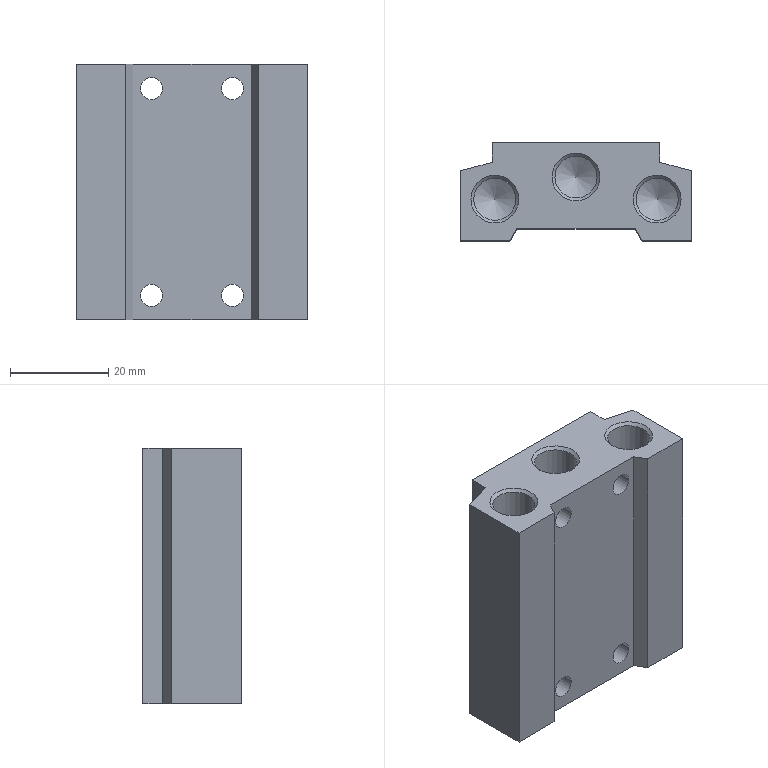Part | NX | 1 solid | 36 faces | box 47 x 20 x 52 mm | volume 37879 mm3 | plane 14 | cone 12 | cylinder 10 | commonest cylinder face diameters 8.566 x6 4.5 x4
STEP:
#1=CARTESIAN_POINT('',(-40.5,20.,0.));
#2=VERTEX_POINT('',#1);
#3=CARTESIAN_POINT('',(-6.5,20.,0.));
#4=VERTEX_POINT('',#3);
#5=CARTESIAN_POINT('',(-6.5,20.,0.));
#6=DIRECTION('',(1.,0.,0.));
#7=VECTOR('',#6,1000.);
#8=LINE('',#5,#7);
#9=EDGE_CURVE('',#2,#4,#8,.T.);
#10=ORIENTED_EDGE('',*,*,#9,.T.);
#11=CARTESIAN_POINT('',(-6.5,20.,-52.));
#12=VERTEX_POINT('',#11);
#13=CARTESIAN_POINT('',(-6.5,20.,0.));
#14=DIRECTION('',(0.,0.,1.));
#15=VECTOR('',#14,1000.);
#16=LINE('',#13,#15);
#17=EDGE_CURVE('',#4,#12,#16,.F.);
#18=ORIENTED_EDGE('',*,*,#17,.T.);
#19=CARTESIAN_POINT('',(-40.5,20.,-52.));
#20=VERTEX_POINT('',#19);
#21=CARTESIAN_POINT('',(-6.5,20.,-52.));
#22=DIRECTION('',(1.,0.,0.));
#23=VECTOR('',#22,1000.);
#24=LINE('',#21,#23);
#25=EDGE_CURVE('',#12,#20,#24,.F.);
#26=ORIENTED_EDGE('',*,*,#25,.T.);
#27=CARTESIAN_POINT('',(-40.5,20.,0.));
#28=DIRECTION('',(0.,0.,1.));
#29=VECTOR('',#28,1000.);
#30=LINE('',#27,#29);
#31=EDGE_CURVE('',#20,#2,#30,.T.);
#32=ORIENTED_EDGE('',*,*,#31,.T.);
#33=EDGE_LOOP('',(#10,#18,#26,#32));
#34=FACE_BOUND('',#33,.T.);
#35=CARTESIAN_POINT('',(-15.25,20.,-7.25));
#36=VERTEX_POINT('',#35);
#37=CARTESIAN_POINT('',(-15.25,20.,-5.));
#38=DIRECTION('',(0.,-1.,0.));
#39=DIRECTION('',(0.,0.,-1.));
#40=AXIS2_PLACEMENT_3D('',#37,#38,#39);
#41=CIRCLE('',#40,2.25);
#42=EDGE_CURVE('',#36,#36,#41,.T.);
#43=ORIENTED_EDGE('',*,*,#42,.T.);
#44=EDGE_LOOP('',(#43));
#45=FACE_BOUND('',#44,.T.);
#46=CARTESIAN_POINT('',(-31.75,20.,-49.25));
#47=VERTEX_POINT('',#46);
#48=CARTESIAN_POINT('',(-31.75,20.,-47.));
#49=DIRECTION('',(0.,-1.,0.));
#50=DIRECTION('',(0.,0.,-1.));
#51=AXIS2_PLACEMENT_3D('',#48,#49,#50);
#52=CIRCLE('',#51,2.25);
#53=EDGE_CURVE('',#47,#47,#52,.T.);
#54=ORIENTED_EDGE('',*,*,#53,.T.);
#55=EDGE_LOOP('',(#54));
#56=FACE_BOUND('',#55,.T.);
#57=CARTESIAN_POINT('',(-31.75,20.,-7.25));
#58=VERTEX_POINT('',#57);
#59=CARTESIAN_POINT('',(-31.75,20.,-5.));
#60=DIRECTION('',(0.,-1.,0.));
#61=DIRECTION('',(0.,0.,-1.));
#62=AXIS2_PLACEMENT_3D('',#59,#60,#61);
#63=CIRCLE('',#62,2.25);
#64=EDGE_CURVE('',#58,#58,#63,.T.);
#65=ORIENTED_EDGE('',*,*,#64,.T.);
#66=EDGE_LOOP('',(#65));
#67=FACE_BOUND('',#66,.T.);
#68=CARTESIAN_POINT('',(-15.25,20.,-49.25));
#69=VERTEX_POINT('',#68);
#70=CARTESIAN_POINT('',(-15.25,20.,-47.));
#71=DIRECTION('',(0.,-1.,0.));
#72=DIRECTION('',(0.,0.,-1.));
#73=AXIS2_PLACEMENT_3D('',#70,#71,#72);
#74=CIRCLE('',#73,2.25);
#75=EDGE_CURVE('',#69,#69,#74,.T.);
#76=ORIENTED_EDGE('',*,*,#75,.T.);
#77=EDGE_LOOP('',(#76));
#78=FACE_BOUND('',#77,.T.);
#79=CARTESIAN_POINT('',(-6.5,20.,0.));
#80=DIRECTION('',(0.,1.,0.));
#81=DIRECTION('',(0.,0.,1.));
#82=AXIS2_PLACEMENT_3D('',#79,#80,#81);
#83=PLANE('',#82);
#84=ADVANCED_FACE('',(#34,#45,#56,#67,#78),#83,.T.);
#85=CARTESIAN_POINT('',(-6.5,16.,0.));
#86=VERTEX_POINT('',#85);
#87=CARTESIAN_POINT('',(-6.5,16.,0.));
#88=DIRECTION('',(0.,1.,0.));
#89=VECTOR('',#88,1000.);
#90=LINE('',#87,#89);
#91=EDGE_CURVE('',#4,#86,#90,.F.);
#92=ORIENTED_EDGE('',*,*,#91,.T.);
#93=CARTESIAN_POINT('',(-6.5,16.,-52.));
#94=VERTEX_POINT('',#93);
#95=CARTESIAN_POINT('',(-6.5,16.,0.));
#96=DIRECTION('',(0.,0.,-1.));
#97=VECTOR('',#96,1000.);
#98=LINE('',#95,#97);
#99=EDGE_CURVE('',#86,#94,#98,.T.);
#100=ORIENTED_EDGE('',*,*,#99,.T.);
#101=CARTESIAN_POINT('',(-6.5,16.,-52.));
#102=DIRECTION('',(0.,1.,0.));
#103=VECTOR('',#102,1000.);
#104=LINE('',#101,#103);
#105=EDGE_CURVE('',#94,#12,#104,.T.);
#106=ORIENTED_EDGE('',*,*,#105,.T.);
#107=ORIENTED_EDGE('',*,*,#17,.F.);
#108=EDGE_LOOP('',(#92,#100,#106,#107));
#109=FACE_BOUND('',#108,.T.);
#110=CARTESIAN_POINT('',(-6.5,16.,0.));
#111=DIRECTION('',(1.,0.,0.));
#112=DIRECTION('',(0.,0.,-1.));
#113=AXIS2_PLACEMENT_3D('',#110,#111,#112);
#114=PLANE('',#113);
#115=ADVANCED_FACE('',(#109),#114,.T.);
#116=CARTESIAN_POINT('',(-40.5,16.,0.));
#117=VERTEX_POINT('',#116);
#118=CARTESIAN_POINT('',(-47.,14.258,0.));
#119=VERTEX_POINT('',#118);
#120=CARTESIAN_POINT('',(-40.5,16.,0.));
#121=DIRECTION('',(-0.9659,-0.2588,0.));
#122=VECTOR('',#121,1000.);
#123=LINE('',#120,#122);
#124=EDGE_CURVE('',#117,#119,#123,.T.);
#125=ORIENTED_EDGE('',*,*,#124,.T.);
#126=CARTESIAN_POINT('',(-47.,0.,0.));
#127=VERTEX_POINT('',#126);
#128=CARTESIAN_POINT('',(-47.,0.,0.));
#129=DIRECTION('',(0.,1.,0.));
#130=VECTOR('',#129,1000.);
#131=LINE('',#128,#130);
#132=EDGE_CURVE('',#119,#127,#131,.F.);
#133=ORIENTED_EDGE('',*,*,#132,.T.);
#134=CARTESIAN_POINT('',(-36.943,0.,0.));
#135=VERTEX_POINT('',#134);
#136=CARTESIAN_POINT('',(0.,0.,0.));
#137=DIRECTION('',(1.,0.,0.));
#138=VECTOR('',#137,1000.);
#139=LINE('',#136,#138);
#140=EDGE_CURVE('',#127,#135,#139,.T.);
#141=ORIENTED_EDGE('',*,*,#140,.T.);
#142=CARTESIAN_POINT('',(-35.5,2.5,0.));
#143=VERTEX_POINT('',#142);
#144=CARTESIAN_POINT('',(-36.943,0.,0.));
#145=DIRECTION('',(0.5,0.866,0.));
#146=VECTOR('',#145,1000.);
#147=LINE('',#144,#146);
#148=EDGE_CURVE('',#135,#143,#147,.T.);
#149=ORIENTED_EDGE('',*,*,#148,.T.);
#150=CARTESIAN_POINT('',(-11.5,2.5,0.));
#151=VERTEX_POINT('',#150);
#152=CARTESIAN_POINT('',(0.,2.5,0.));
#153=DIRECTION('',(1.,0.,0.));
#154=VECTOR('',#153,1000.);
#155=LINE('',#152,#154);
#156=EDGE_CURVE('',#143,#151,#155,.T.);
#157=ORIENTED_EDGE('',*,*,#156,.T.);
#158=CARTESIAN_POINT('',(-10.057,0.,0.));
#159=VERTEX_POINT('',#158);
#160=CARTESIAN_POINT('',(-11.5,2.5,0.));
#161=DIRECTION('',(0.5,-0.866,0.));
#162=VECTOR('',#161,1000.);
#163=LINE('',#160,#162);
#164=EDGE_CURVE('',#151,#159,#163,.T.);
#165=ORIENTED_EDGE('',*,*,#164,.T.);
#166=CARTESIAN_POINT('',(0.,0.,0.));
#167=VERTEX_POINT('',#166);
#168=CARTESIAN_POINT('',(0.,0.,0.));
#169=DIRECTION('',(1.,0.,0.));
#170=VECTOR('',#169,1000.);
#171=LINE('',#168,#170);
#172=EDGE_CURVE('',#159,#167,#171,.T.);
#173=ORIENTED_EDGE('',*,*,#172,.T.);
#174=CARTESIAN_POINT('',(0.,14.258,0.));
#175=VERTEX_POINT('',#174);
#176=CARTESIAN_POINT('',(0.,0.,0.));
#177=DIRECTION('',(0.,1.,0.));
#178=VECTOR('',#177,1000.);
#179=LINE('',#176,#178);
#180=EDGE_CURVE('',#167,#175,#179,.T.);
#181=ORIENTED_EDGE('',*,*,#180,.T.);
#182=CARTESIAN_POINT('',(0.,14.258,0.));
#183=DIRECTION('',(-0.9659,0.2588,0.));
#184=VECTOR('',#183,1000.);
#185=LINE('',#182,#184);
#186=EDGE_CURVE('',#175,#86,#185,.T.);
#187=ORIENTED_EDGE('',*,*,#186,.T.);
#188=ORIENTED_EDGE('',*,*,#91,.F.);
#189=ORIENTED_EDGE('',*,*,#9,.F.);
#190=CARTESIAN_POINT('',(-40.5,0.,0.));
#191=DIRECTION('',(0.,1.,0.));
#192=VECTOR('',#191,1000.);
#193=LINE('',#190,#192);
#194=EDGE_CURVE('',#2,#117,#193,.F.);
#195=ORIENTED_EDGE('',*,*,#194,.T.);
#196=EDGE_LOOP('',(#125,#133,#141,#149,#157,#165,#173,#181,#187,#188,#189,#195));
#197=FACE_BOUND('',#196,.T.);
#198=CARTESIAN_POINT('',(-2.136,8.5,0.));
#199=VERTEX_POINT('',#198);
#200=CARTESIAN_POINT('',(-7.,8.5,0.));
#201=DIRECTION('',(0.,0.,1.));
#202=DIRECTION('',(1.,0.,0.));
#203=AXIS2_PLACEMENT_3D('',#200,#201,#202);
#204=CIRCLE('',#203,4.864);
#205=EDGE_CURVE('',#199,#199,#204,.F.);
#206=ORIENTED_EDGE('',*,*,#205,.T.);
#207=EDGE_LOOP('',(#206));
#208=FACE_BOUND('',#207,.T.);
#209=CARTESIAN_POINT('',(-18.636,13.,0.));
#210=VERTEX_POINT('',#209);
#211=CARTESIAN_POINT('',(-23.5,13.,0.));
#212=DIRECTION('',(0.,0.,1.));
#213=DIRECTION('',(1.,0.,0.));
#214=AXIS2_PLACEMENT_3D('',#211,#212,#213);
#215=CIRCLE('',#214,4.864);
#216=EDGE_CURVE('',#210,#210,#215,.F.);
#217=ORIENTED_EDGE('',*,*,#216,.T.);
#218=EDGE_LOOP('',(#217));
#219=FACE_BOUND('',#218,.T.);
#220=CARTESIAN_POINT('',(-35.136,8.5,0.));
#221=VERTEX_POINT('',#220);
#222=CARTESIAN_POINT('',(-40.,8.5,0.));
#223=DIRECTION('',(0.,0.,1.));
#224=DIRECTION('',(1.,0.,0.));
#225=AXIS2_PLACEMENT_3D('',#222,#223,#224);
#226=CIRCLE('',#225,4.864);
#227=EDGE_CURVE('',#221,#221,#226,.F.);
#228=ORIENTED_EDGE('',*,*,#227,.T.);
#229=EDGE_LOOP('',(#228));
#230=FACE_BOUND('',#229,.T.);
#231=CARTESIAN_POINT('',(0.,0.,0.));
#232=DIRECTION('',(0.,0.,1.));
#233=DIRECTION('',(1.,0.,0.));
#234=AXIS2_PLACEMENT_3D('',#231,#232,#233);
#235=PLANE('',#234);
#236=ADVANCED_FACE('',(#197,#208,#219,#230),#235,.T.);
#237=ORIENTED_EDGE('',*,*,#194,.F.);
#238=ORIENTED_EDGE('',*,*,#31,.F.);
#239=CARTESIAN_POINT('',(-40.5,16.,-52.));
#240=VERTEX_POINT('',#239);
#241=CARTESIAN_POINT('',(-40.5,20.,-52.));
#242=DIRECTION('',(0.,1.,0.));
#243=VECTOR('',#242,1000.);
#244=LINE('',#241,#243);
#245=EDGE_CURVE('',#20,#240,#244,.F.);
#246=ORIENTED_EDGE('',*,*,#245,.T.);
#247=CARTESIAN_POINT('',(-40.5,16.,0.));
#248=DIRECTION('',(0.,0.,1.));
#249=VECTOR('',#248,1000.);
#250=LINE('',#247,#249);
#251=EDGE_CURVE('',#240,#117,#250,.T.);
#252=ORIENTED_EDGE('',*,*,#251,.T.);
#253=EDGE_LOOP('',(#237,#238,#246,#252));
#254=FACE_BOUND('',#253,.T.);
#255=CARTESIAN_POINT('',(-40.5,20.,0.));
#256=DIRECTION('',(-1.,0.,0.));
#257=DIRECTION('',(0.,0.,1.));
#258=AXIS2_PLACEMENT_3D('',#255,#256,#257);
#259=PLANE('',#258);
#260=ADVANCED_FACE('',(#254),#259,.T.);
#261=CARTESIAN_POINT('',(-47.,0.,-52.));
#262=VERTEX_POINT('',#261);
#263=CARTESIAN_POINT('',(-36.943,0.,-52.));
#264=VERTEX_POINT('',#263);
#265=CARTESIAN_POINT('',(0.,0.,-52.));
#266=DIRECTION('',(1.,0.,0.));
#267=VECTOR('',#266,1000.);
#268=LINE('',#265,#267);
#269=EDGE_CURVE('',#262,#264,#268,.T.);
#270=ORIENTED_EDGE('',*,*,#269,.F.);
#271=CARTESIAN_POINT('',(-47.,14.258,-52.));
#272=VERTEX_POINT('',#271);
#273=CARTESIAN_POINT('',(-47.,0.,-52.));
#274=DIRECTION('',(0.,1.,0.));
#275=VECTOR('',#274,1000.);
#276=LINE('',#273,#275);
#277=EDGE_CURVE('',#272,#262,#276,.F.);
#278=ORIENTED_EDGE('',*,*,#277,.F.);
#279=CARTESIAN_POINT('',(-40.5,16.,-52.));
#280=DIRECTION('',(-0.9659,-0.2588,0.));
#281=VECTOR('',#280,1000.);
#282=LINE('',#279,#281);
#283=EDGE_CURVE('',#240,#272,#282,.T.);
#284=ORIENTED_EDGE('',*,*,#283,.F.);
#285=ORIENTED_EDGE('',*,*,#245,.F.);
#286=ORIENTED_EDGE('',*,*,#25,.F.);
#287=ORIENTED_EDGE('',*,*,#105,.F.);
#288=CARTESIAN_POINT('',(0.,14.258,-52.));
#289=VERTEX_POINT('',#288);
#290=CARTESIAN_POINT('',(0.,14.258,-52.));
#291=DIRECTION('',(-0.9659,0.2588,0.));
#292=VECTOR('',#291,1000.);
#293=LINE('',#290,#292);
#294=EDGE_CURVE('',#289,#94,#293,.T.);
#295=ORIENTED_EDGE('',*,*,#294,.F.);
#296=CARTESIAN_POINT('',(0.,0.,-52.));
#297=VERTEX_POINT('',#296);
#298=CARTESIAN_POINT('',(0.,0.,-52.));
#299=DIRECTION('',(0.,1.,0.));
#300=VECTOR('',#299,1000.);
#301=LINE('',#298,#300);
#302=EDGE_CURVE('',#297,#289,#301,.T.);
#303=ORIENTED_EDGE('',*,*,#302,.F.);
#304=CARTESIAN_POINT('',(-10.057,0.,-52.));
#305=VERTEX_POINT('',#304);
#306=CARTESIAN_POINT('',(0.,0.,-52.));
#307=DIRECTION('',(1.,0.,0.));
#308=VECTOR('',#307,1000.);
#309=LINE('',#306,#308);
#310=EDGE_CURVE('',#305,#297,#309,.T.);
#311=ORIENTED_EDGE('',*,*,#310,.F.);
#312=CARTESIAN_POINT('',(-11.5,2.5,-52.));
#313=VERTEX_POINT('',#312);
#314=CARTESIAN_POINT('',(-11.5,2.5,-52.));
#315=DIRECTION('',(0.5,-0.866,0.));
#316=VECTOR('',#315,1000.);
#317=LINE('',#314,#316);
#318=EDGE_CURVE('',#313,#305,#317,.T.);
#319=ORIENTED_EDGE('',*,*,#318,.F.);
#320=CARTESIAN_POINT('',(-35.5,2.5,-52.));
#321=VERTEX_POINT('',#320);
#322=CARTESIAN_POINT('',(0.,2.5,-52.));
#323=DIRECTION('',(1.,0.,0.));
#324=VECTOR('',#323,1000.);
#325=LINE('',#322,#324);
#326=EDGE_CURVE('',#321,#313,#325,.T.);
#327=ORIENTED_EDGE('',*,*,#326,.F.);
#328=CARTESIAN_POINT('',(-36.943,0.,-52.));
#329=DIRECTION('',(0.5,0.866,0.));
#330=VECTOR('',#329,1000.);
#331=LINE('',#328,#330);
#332=EDGE_CURVE('',#264,#321,#331,.T.);
#333=ORIENTED_EDGE('',*,*,#332,.F.);
#334=EDGE_LOOP('',(#270,#278,#284,#285,#286,#287,#295,#303,#311,#319,#327,#333));
#335=FACE_BOUND('',#334,.T.);
#336=CARTESIAN_POINT('',(-11.864,8.5,-52.));
#337=VERTEX_POINT('',#336);
#338=CARTESIAN_POINT('',(-7.,8.5,-52.));
#339=DIRECTION('',(0.,0.,-1.));
#340=DIRECTION('',(-1.,0.,0.));
#341=AXIS2_PLACEMENT_3D('',#338,#339,#340);
#342=CIRCLE('',#341,4.864);
#343=EDGE_CURVE('',#337,#337,#342,.T.);
#344=ORIENTED_EDGE('',*,*,#343,.F.);
#345=EDGE_LOOP('',(#344));
#346=FACE_BOUND('',#345,.T.);
#347=CARTESIAN_POINT('',(-28.364,13.,-52.));
#348=VERTEX_POINT('',#347);
#349=CARTESIAN_POINT('',(-23.5,13.,-52.));
#350=DIRECTION('',(0.,0.,-1.));
#351=DIRECTION('',(-1.,0.,0.));
#352=AXIS2_PLACEMENT_3D('',#349,#350,#351);
#353=CIRCLE('',#352,4.864);
#354=EDGE_CURVE('',#348,#348,#353,.T.);
#355=ORIENTED_EDGE('',*,*,#354,.F.);
#356=EDGE_LOOP('',(#355));
#357=FACE_BOUND('',#356,.T.);
#358=CARTESIAN_POINT('',(-44.864,8.5,-52.));
#359=VERTEX_POINT('',#358);
#360=CARTESIAN_POINT('',(-40.,8.5,-52.));
#361=DIRECTION('',(0.,0.,-1.));
#362=DIRECTION('',(-1.,0.,0.));
#363=AXIS2_PLACEMENT_3D('',#360,#361,#362);
#364=CIRCLE('',#363,4.864);
#365=EDGE_CURVE('',#359,#359,#364,.T.);
#366=ORIENTED_EDGE('',*,*,#365,.F.);
#367=EDGE_LOOP('',(#366));
#368=FACE_BOUND('',#367,.T.);
#369=CARTESIAN_POINT('',(0.,0.,-52.));
#370=DIRECTION('',(0.,0.,1.));
#371=DIRECTION('',(1.,0.,0.));
#372=AXIS2_PLACEMENT_3D('',#369,#370,#371);
#373=PLANE('',#372);
#374=ADVANCED_FACE('',(#335,#346,#357,#368),#373,.F.);
#375=ORIENTED_EDGE('',*,*,#42,.F.);
#376=EDGE_LOOP('',(#375));
#377=FACE_BOUND('',#376,.T.);
#378=CARTESIAN_POINT('',(-15.25,2.5,-7.25));
#379=VERTEX_POINT('',#378);
#380=CARTESIAN_POINT('',(-15.25,2.5,-5.));
#381=DIRECTION('',(0.,-1.,0.));
#382=DIRECTION('',(0.,0.,-1.));
#383=AXIS2_PLACEMENT_3D('',#380,#381,#382);
#384=CIRCLE('',#383,2.25);
#385=EDGE_CURVE('',#379,#379,#384,.F.);
#386=ORIENTED_EDGE('',*,*,#385,.F.);
#387=EDGE_LOOP('',(#386));
#388=FACE_BOUND('',#387,.T.);
#389=CARTESIAN_POINT('',(-15.25,11.,-5.));
#390=DIRECTION('',(0.,-1.,0.));
#391=DIRECTION('',(0.,0.,-1.));
#392=AXIS2_PLACEMENT_3D('',#389,#390,#391);
#393=CYLINDRICAL_SURFACE('',#392,2.25);
#394=ADVANCED_FACE('',(#377,#388),#393,.F.);
#395=ORIENTED_EDGE('',*,*,#53,.F.);
#396=EDGE_LOOP('',(#395));
#397=FACE_BOUND('',#396,.T.);
#398=CARTESIAN_POINT('',(-31.75,2.5,-49.25));
#399=VERTEX_POINT('',#398);
#400=CARTESIAN_POINT('',(-31.75,2.5,-47.));
#401=DIRECTION('',(0.,-1.,0.));
#402=DIRECTION('',(0.,0.,-1.));
#403=AXIS2_PLACEMENT_3D('',#400,#401,#402);
#404=CIRCLE('',#403,2.25);
#405=EDGE_CURVE('',#399,#399,#404,.F.);
#406=ORIENTED_EDGE('',*,*,#405,.F.);
#407=EDGE_LOOP('',(#406));
#408=FACE_BOUND('',#407,.T.);
#409=CARTESIAN_POINT('',(-31.75,11.,-47.));
#410=DIRECTION('',(0.,-1.,0.));
#411=DIRECTION('',(0.,0.,-1.));
#412=AXIS2_PLACEMENT_3D('',#409,#410,#411);
#413=CYLINDRICAL_SURFACE('',#412,2.25);
#414=ADVANCED_FACE('',(#397,#408),#413,.F.);
#415=ORIENTED_EDGE('',*,*,#64,.F.);
#416=EDGE_LOOP('',(#415));
#417=FACE_BOUND('',#416,.T.);
#418=CARTESIAN_POINT('',(-31.75,2.5,-7.25));
#419=VERTEX_POINT('',#418);
#420=CARTESIAN_POINT('',(-31.75,2.5,-5.));
#421=DIRECTION('',(0.,-1.,0.));
#422=DIRECTION('',(0.,0.,-1.));
#423=AXIS2_PLACEMENT_3D('',#420,#421,#422);
#424=CIRCLE('',#423,2.25);
#425=EDGE_CURVE('',#419,#419,#424,.F.);
#426=ORIENTED_EDGE('',*,*,#425,.F.);
#427=EDGE_LOOP('',(#426));
#428=FACE_BOUND('',#427,.T.);
#429=CARTESIAN_POINT('',(-31.75,11.,-5.));
#430=DIRECTION('',(0.,-1.,0.));
#431=DIRECTION('',(0.,0.,-1.));
#432=AXIS2_PLACEMENT_3D('',#429,#430,#431);
#433=CYLINDRICAL_SURFACE('',#432,2.25);
#434=ADVANCED_FACE('',(#417,#428),#433,.F.);
#435=ORIENTED_EDGE('',*,*,#75,.F.);
#436=EDGE_LOOP('',(#435));
#437=FACE_BOUND('',#436,.T.);
#438=CARTESIAN_POINT('',(-15.25,2.5,-49.25));
#439=VERTEX_POINT('',#438);
#440=CARTESIAN_POINT('',(-15.25,2.5,-47.));
#441=DIRECTION('',(0.,-1.,0.));
#442=DIRECTION('',(0.,0.,-1.));
#443=AXIS2_PLACEMENT_3D('',#440,#441,#442);
#444=CIRCLE('',#443,2.25);
#445=EDGE_CURVE('',#439,#439,#444,.F.);
#446=ORIENTED_EDGE('',*,*,#445,.F.);
#447=EDGE_LOOP('',(#446));
#448=FACE_BOUND('',#447,.T.);
#449=CARTESIAN_POINT('',(-15.25,11.,-47.));
#450=DIRECTION('',(0.,-1.,0.));
#451=DIRECTION('',(0.,0.,-1.));
#452=AXIS2_PLACEMENT_3D('',#449,#450,#451);
#453=CYLINDRICAL_SURFACE('',#452,2.25);
#454=ADVANCED_FACE('',(#437,#448),#453,.F.);
#455=ORIENTED_EDGE('',*,*,#186,.F.);
#456=CARTESIAN_POINT('',(0.,14.258,0.));
#457=DIRECTION('',(0.,0.,1.));
#458=VECTOR('',#457,1000.);
#459=LINE('',#456,#458);
#460=EDGE_CURVE('',#175,#289,#459,.F.);
#461=ORIENTED_EDGE('',*,*,#460,.T.);
#462=ORIENTED_EDGE('',*,*,#294,.T.);
#463=ORIENTED_EDGE('',*,*,#99,.F.);
#464=EDGE_LOOP('',(#455,#461,#462,#463));
#465=FACE_BOUND('',#464,.T.);
#466=CARTESIAN_POINT('',(0.,14.258,0.));
#467=DIRECTION('',(0.2588,0.9659,0.));
#468=DIRECTION('',(-0.9659,0.2588,0.));
#469=AXIS2_PLACEMENT_3D('',#466,#467,#468);
#470=PLANE('',#469);
#471=ADVANCED_FACE('',(#465),#470,.T.);
#472=ORIENTED_EDGE('',*,*,#132,.F.);
#473=CARTESIAN_POINT('',(-47.,14.258,0.));
#474=DIRECTION('',(0.,0.,1.));
#475=VECTOR('',#474,1000.);
#476=LINE('',#473,#475);
#477=EDGE_CURVE('',#119,#272,#476,.F.);
#478=ORIENTED_EDGE('',*,*,#477,.T.);
#479=ORIENTED_EDGE('',*,*,#277,.T.);
#480=CARTESIAN_POINT('',(-47.,0.,0.));
#481=DIRECTION('',(0.,0.,1.));
#482=VECTOR('',#481,1000.);
#483=LINE('',#480,#482);
#484=EDGE_CURVE('',#262,#127,#483,.T.);
#485=ORIENTED_EDGE('',*,*,#484,.T.);
#486=EDGE_LOOP('',(#472,#478,#479,#485));
#487=FACE_BOUND('',#486,.T.);
#488=CARTESIAN_POINT('',(-47.,14.258,0.));
#489=DIRECTION('',(-1.,0.,0.));
#490=DIRECTION('',(0.,0.,1.));
#491=AXIS2_PLACEMENT_3D('',#488,#489,#490);
#492=PLANE('',#491);
#493=ADVANCED_FACE('',(#487),#492,.T.);
#494=ORIENTED_EDGE('',*,*,#124,.F.);
#495=ORIENTED_EDGE('',*,*,#251,.F.);
#496=ORIENTED_EDGE('',*,*,#283,.T.);
#497=ORIENTED_EDGE('',*,*,#477,.F.);
#498=EDGE_LOOP('',(#494,#495,#496,#497));
#499=FACE_BOUND('',#498,.T.);
#500=CARTESIAN_POINT('',(-40.5,16.,0.));
#501=DIRECTION('',(-0.2588,0.9659,0.));
#502=DIRECTION('',(-0.9659,-0.2588,0.));
#503=AXIS2_PLACEMENT_3D('',#500,#501,#502);
#504=PLANE('',#503);
#505=ADVANCED_FACE('',(#499),#504,.T.);
#506=ORIENTED_EDGE('',*,*,#180,.F.);
#507=CARTESIAN_POINT('',(0.,0.,0.));
#508=DIRECTION('',(0.,0.,-1.));
#509=VECTOR('',#508,1000.);
#510=LINE('',#507,#509);
#511=EDGE_CURVE('',#167,#297,#510,.T.);
#512=ORIENTED_EDGE('',*,*,#511,.T.);
#513=ORIENTED_EDGE('',*,*,#302,.T.);
#514=ORIENTED_EDGE('',*,*,#460,.F.);
#515=EDGE_LOOP('',(#506,#512,#513,#514));
#516=FACE_BOUND('',#515,.T.);
#517=CARTESIAN_POINT('',(0.,0.,0.));
#518=DIRECTION('',(1.,0.,0.));
#519=DIRECTION('',(0.,0.,-1.));
#520=AXIS2_PLACEMENT_3D('',#517,#518,#519);
#521=PLANE('',#520);
#522=ADVANCED_FACE('',(#516),#521,.T.);
#523=ORIENTED_EDGE('',*,*,#172,.F.);
#524=CARTESIAN_POINT('',(-10.057,0.,0.));
#525=DIRECTION('',(0.,0.,-1.));
#526=VECTOR('',#525,1000.);
#527=LINE('',#524,#526);
#528=EDGE_CURVE('',#159,#305,#527,.T.);
#529=ORIENTED_EDGE('',*,*,#528,.T.);
#530=ORIENTED_EDGE('',*,*,#310,.T.);
#531=ORIENTED_EDGE('',*,*,#511,.F.);
#532=EDGE_LOOP('',(#523,#529,#530,#531));
#533=FACE_BOUND('',#532,.T.);
#534=CARTESIAN_POINT('',(-10.057,0.,0.));
#535=DIRECTION('',(0.,-1.,0.));
#536=DIRECTION('',(0.,0.,-1.));
#537=AXIS2_PLACEMENT_3D('',#534,#535,#536);
#538=PLANE('',#537);
#539=ADVANCED_FACE('',(#533),#538,.T.);
#540=ORIENTED_EDGE('',*,*,#164,.F.);
#541=CARTESIAN_POINT('',(-11.5,2.5,0.));
#542=DIRECTION('',(0.,0.,1.));
#543=VECTOR('',#542,1000.);
#544=LINE('',#541,#543);
#545=EDGE_CURVE('',#151,#313,#544,.F.);
#546=ORIENTED_EDGE('',*,*,#545,.T.);
#547=ORIENTED_EDGE('',*,*,#318,.T.);
#548=ORIENTED_EDGE('',*,*,#528,.F.);
#549=EDGE_LOOP('',(#540,#546,#547,#548));
#550=FACE_BOUND('',#549,.T.);
#551=CARTESIAN_POINT('',(-11.5,2.5,0.));
#552=DIRECTION('',(-0.866,-0.5,0.));
#553=DIRECTION('',(0.5,-0.866,0.));
#554=AXIS2_PLACEMENT_3D('',#551,#552,#553);
#555=PLANE('',#554);
#556=ADVANCED_FACE('',(#550),#555,.T.);
#557=ORIENTED_EDGE('',*,*,#156,.F.);
#558=CARTESIAN_POINT('',(-35.5,2.5,0.));
#559=DIRECTION('',(0.,0.,-1.));
#560=VECTOR('',#559,1000.);
#561=LINE('',#558,#560);
#562=EDGE_CURVE('',#143,#321,#561,.T.);
#563=ORIENTED_EDGE('',*,*,#562,.T.);
#564=ORIENTED_EDGE('',*,*,#326,.T.);
#565=ORIENTED_EDGE('',*,*,#545,.F.);
#566=EDGE_LOOP('',(#557,#563,#564,#565));
#567=FACE_BOUND('',#566,.T.);
#568=ORIENTED_EDGE('',*,*,#385,.T.);
#569=EDGE_LOOP('',(#568));
#570=FACE_BOUND('',#569,.T.);
#571=ORIENTED_EDGE('',*,*,#405,.T.);
#572=EDGE_LOOP('',(#571));
#573=FACE_BOUND('',#572,.T.);
#574=ORIENTED_EDGE('',*,*,#425,.T.);
#575=EDGE_LOOP('',(#574));
#576=FACE_BOUND('',#575,.T.);
#577=ORIENTED_EDGE('',*,*,#445,.T.);
#578=EDGE_LOOP('',(#577));
#579=FACE_BOUND('',#578,.T.);
#580=CARTESIAN_POINT('',(-35.5,2.5,0.));
#581=DIRECTION('',(0.,-1.,0.));
#582=DIRECTION('',(0.,0.,-1.));
#583=AXIS2_PLACEMENT_3D('',#580,#581,#582);
#584=PLANE('',#583);
#585=ADVANCED_FACE('',(#567,#570,#573,#576,#579),#584,.T.);
#586=ORIENTED_EDGE('',*,*,#148,.F.);
#587=CARTESIAN_POINT('',(-36.943,0.,0.));
#588=DIRECTION('',(0.,0.,1.));
#589=VECTOR('',#588,1000.);
#590=LINE('',#587,#589);
#591=EDGE_CURVE('',#135,#264,#590,.F.);
#592=ORIENTED_EDGE('',*,*,#591,.T.);
#593=ORIENTED_EDGE('',*,*,#332,.T.);
#594=ORIENTED_EDGE('',*,*,#562,.F.);
#595=EDGE_LOOP('',(#586,#592,#593,#594));
#596=FACE_BOUND('',#595,.T.);
#597=CARTESIAN_POINT('',(-36.943,0.,0.));
#598=DIRECTION('',(0.866,-0.5,0.));
#599=DIRECTION('',(0.5,0.866,0.));
#600=AXIS2_PLACEMENT_3D('',#597,#598,#599);
#601=PLANE('',#600);
#602=ADVANCED_FACE('',(#596),#601,.T.);
#603=ORIENTED_EDGE('',*,*,#140,.F.);
#604=ORIENTED_EDGE('',*,*,#484,.F.);
#605=ORIENTED_EDGE('',*,*,#269,.T.);
#606=ORIENTED_EDGE('',*,*,#591,.F.);
#607=EDGE_LOOP('',(#603,#604,#605,#606));
#608=FACE_BOUND('',#607,.T.);
#609=CARTESIAN_POINT('',(-47.,0.,0.));
#610=DIRECTION('',(0.,-1.,0.));
#611=DIRECTION('',(0.,0.,-1.));
#612=AXIS2_PLACEMENT_3D('',#609,#610,#611);
#613=PLANE('',#612);
#614=ADVANCED_FACE('',(#608),#613,.T.);
#615=ORIENTED_EDGE('',*,*,#205,.F.);
#616=EDGE_LOOP('',(#615));
#617=FACE_BOUND('',#616,.T.);
#618=CARTESIAN_POINT('',(-2.717,8.5,-0.581));
#619=VERTEX_POINT('',#618);
#620=CARTESIAN_POINT('',(-7.,8.5,-0.581));
#621=DIRECTION('',(0.,0.,1.));
#622=DIRECTION('',(1.,0.,0.));
#623=AXIS2_PLACEMENT_3D('',#620,#621,#622);
#624=CIRCLE('',#623,4.283);
#625=EDGE_CURVE('',#619,#619,#624,.T.);
#626=ORIENTED_EDGE('',*,*,#625,.F.);
#627=EDGE_LOOP('',(#626));
#628=FACE_BOUND('',#627,.T.);
#629=CARTESIAN_POINT('',(-7.,8.5,0.));
#630=DIRECTION('',(0.,0.,1.));
#631=DIRECTION('',(1.,0.,0.));
#632=AXIS2_PLACEMENT_3D('',#629,#630,#631);
#633=CONICAL_SURFACE('',#632,4.864,0.7854);
#634=ADVANCED_FACE('',(#617,#628),#633,.F.);
#635=ORIENTED_EDGE('',*,*,#216,.F.);
#636=EDGE_LOOP('',(#635));
#637=FACE_BOUND('',#636,.T.);
#638=CARTESIAN_POINT('',(-19.217,13.,-0.581));
#639=VERTEX_POINT('',#638);
#640=CARTESIAN_POINT('',(-23.5,13.,-0.581));
#641=DIRECTION('',(0.,0.,1.));
#642=DIRECTION('',(1.,0.,0.));
#643=AXIS2_PLACEMENT_3D('',#640,#641,#642);
#644=CIRCLE('',#643,4.283);
#645=EDGE_CURVE('',#639,#639,#644,.T.);
#646=ORIENTED_EDGE('',*,*,#645,.F.);
#647=EDGE_LOOP('',(#646));
#648=FACE_BOUND('',#647,.T.);
#649=CARTESIAN_POINT('',(-23.5,13.,0.));
#650=DIRECTION('',(0.,0.,1.));
#651=DIRECTION('',(1.,0.,0.));
#652=AXIS2_PLACEMENT_3D('',#649,#650,#651);
#653=CONICAL_SURFACE('',#652,4.864,0.7854);
#654=ADVANCED_FACE('',(#637,#648),#653,.F.);
#655=ORIENTED_EDGE('',*,*,#227,.F.);
#656=EDGE_LOOP('',(#655));
#657=FACE_BOUND('',#656,.T.);
#658=CARTESIAN_POINT('',(-35.717,8.5,-0.581));
#659=VERTEX_POINT('',#658);
#660=CARTESIAN_POINT('',(-40.,8.5,-0.581));
#661=DIRECTION('',(0.,0.,1.));
#662=DIRECTION('',(1.,0.,0.));
#663=AXIS2_PLACEMENT_3D('',#660,#661,#662);
#664=CIRCLE('',#663,4.283);
#665=EDGE_CURVE('',#659,#659,#664,.T.);
#666=ORIENTED_EDGE('',*,*,#665,.F.);
#667=EDGE_LOOP('',(#666));
#668=FACE_BOUND('',#667,.T.);
#669=CARTESIAN_POINT('',(-40.,8.5,0.));
#670=DIRECTION('',(0.,0.,1.));
#671=DIRECTION('',(1.,0.,0.));
#672=AXIS2_PLACEMENT_3D('',#669,#670,#671);
#673=CONICAL_SURFACE('',#672,4.864,0.7854);
#674=ADVANCED_FACE('',(#657,#668),#673,.F.);
#675=CARTESIAN_POINT('',(-2.717,8.5,-51.419));
#676=VERTEX_POINT('',#675);
#677=CARTESIAN_POINT('',(-7.,8.5,-51.419));
#678=DIRECTION('',(0.,0.,-1.));
#679=DIRECTION('',(1.,0.,0.));
#680=AXIS2_PLACEMENT_3D('',#677,#678,#679);
#681=CIRCLE('',#680,4.283);
#682=EDGE_CURVE('',#676,#676,#681,.T.);
#683=ORIENTED_EDGE('',*,*,#682,.F.);
#684=EDGE_LOOP('',(#683));
#685=FACE_BOUND('',#684,.T.);
#686=ORIENTED_EDGE('',*,*,#343,.T.);
#687=EDGE_LOOP('',(#686));
#688=FACE_BOUND('',#687,.T.);
#689=CARTESIAN_POINT('',(-7.,8.5,-52.));
#690=DIRECTION('',(0.,0.,-1.));
#691=DIRECTION('',(-1.,0.,0.));
#692=AXIS2_PLACEMENT_3D('',#689,#690,#691);
#693=CONICAL_SURFACE('',#692,4.864,0.7854);
#694=ADVANCED_FACE('',(#685,#688),#693,.F.);
#695=CARTESIAN_POINT('',(-19.217,13.,-51.419));
#696=VERTEX_POINT('',#695);
#697=CARTESIAN_POINT('',(-23.5,13.,-51.419));
#698=DIRECTION('',(0.,0.,-1.));
#699=DIRECTION('',(1.,0.,0.));
#700=AXIS2_PLACEMENT_3D('',#697,#698,#699);
#701=CIRCLE('',#700,4.283);
#702=EDGE_CURVE('',#696,#696,#701,.T.);
#703=ORIENTED_EDGE('',*,*,#702,.F.);
#704=EDGE_LOOP('',(#703));
#705=FACE_BOUND('',#704,.T.);
#706=ORIENTED_EDGE('',*,*,#354,.T.);
#707=EDGE_LOOP('',(#706));
#708=FACE_BOUND('',#707,.T.);
#709=CARTESIAN_POINT('',(-23.5,13.,-52.));
#710=DIRECTION('',(0.,0.,-1.));
#711=DIRECTION('',(-1.,0.,0.));
#712=AXIS2_PLACEMENT_3D('',#709,#710,#711);
#713=CONICAL_SURFACE('',#712,4.864,0.7854);
#714=ADVANCED_FACE('',(#705,#708),#713,.F.);
#715=CARTESIAN_POINT('',(-35.717,8.5,-51.419));
#716=VERTEX_POINT('',#715);
#717=CARTESIAN_POINT('',(-40.,8.5,-51.419));
#718=DIRECTION('',(0.,0.,-1.));
#719=DIRECTION('',(1.,0.,0.));
#720=AXIS2_PLACEMENT_3D('',#717,#718,#719);
#721=CIRCLE('',#720,4.283);
#722=EDGE_CURVE('',#716,#716,#721,.T.);
#723=ORIENTED_EDGE('',*,*,#722,.F.);
#724=EDGE_LOOP('',(#723));
#725=FACE_BOUND('',#724,.T.);
#726=ORIENTED_EDGE('',*,*,#365,.T.);
#727=EDGE_LOOP('',(#726));
#728=FACE_BOUND('',#727,.T.);
#729=CARTESIAN_POINT('',(-40.,8.5,-52.));
#730=DIRECTION('',(0.,0.,-1.));
#731=DIRECTION('',(-1.,0.,0.));
#732=AXIS2_PLACEMENT_3D('',#729,#730,#731);
#733=CONICAL_SURFACE('',#732,4.864,0.7854);
#734=ADVANCED_FACE('',(#725,#728),#733,.F.);
#735=ORIENTED_EDGE('',*,*,#625,.T.);
#736=EDGE_LOOP('',(#735));
#737=FACE_BOUND('',#736,.T.);
#738=CARTESIAN_POINT('',(-2.717,8.5,-9.));
#739=VERTEX_POINT('',#738);
#740=CARTESIAN_POINT('',(-7.,8.5,-9.));
#741=DIRECTION('',(0.,0.,1.));
#742=DIRECTION('',(1.,0.,0.));
#743=AXIS2_PLACEMENT_3D('',#740,#741,#742);
#744=CIRCLE('',#743,4.283);
#745=EDGE_CURVE('',#739,#739,#744,.T.);
#746=ORIENTED_EDGE('',*,*,#745,.F.);
#747=EDGE_LOOP('',(#746));
#748=FACE_BOUND('',#747,.T.);
#749=CARTESIAN_POINT('',(-7.,8.5,-4.79));
#750=DIRECTION('',(0.,0.,1.));
#751=DIRECTION('',(1.,0.,0.));
#752=AXIS2_PLACEMENT_3D('',#749,#750,#751);
#753=CYLINDRICAL_SURFACE('',#752,4.283);
#754=ADVANCED_FACE('',(#737,#748),#753,.F.);
#755=ORIENTED_EDGE('',*,*,#645,.T.);
#756=EDGE_LOOP('',(#755));
#757=FACE_BOUND('',#756,.T.);
#758=CARTESIAN_POINT('',(-19.217,13.,-9.));
#759=VERTEX_POINT('',#758);
#760=CARTESIAN_POINT('',(-23.5,13.,-9.));
#761=DIRECTION('',(0.,0.,1.));
#762=DIRECTION('',(1.,0.,0.));
#763=AXIS2_PLACEMENT_3D('',#760,#761,#762);
#764=CIRCLE('',#763,4.283);
#765=EDGE_CURVE('',#759,#759,#764,.T.);
#766=ORIENTED_EDGE('',*,*,#765,.F.);
#767=EDGE_LOOP('',(#766));
#768=FACE_BOUND('',#767,.T.);
#769=CARTESIAN_POINT('',(-23.5,13.,-4.79));
#770=DIRECTION('',(0.,0.,1.));
#771=DIRECTION('',(1.,0.,0.));
#772=AXIS2_PLACEMENT_3D('',#769,#770,#771);
#773=CYLINDRICAL_SURFACE('',#772,4.283);
#774=ADVANCED_FACE('',(#757,#768),#773,.F.);
#775=ORIENTED_EDGE('',*,*,#665,.T.);
#776=EDGE_LOOP('',(#775));
#777=FACE_BOUND('',#776,.T.);
#778=CARTESIAN_POINT('',(-35.717,8.5,-9.));
#779=VERTEX_POINT('',#778);
#780=CARTESIAN_POINT('',(-40.,8.5,-9.));
#781=DIRECTION('',(0.,0.,1.));
#782=DIRECTION('',(1.,0.,0.));
#783=AXIS2_PLACEMENT_3D('',#780,#781,#782);
#784=CIRCLE('',#783,4.283);
#785=EDGE_CURVE('',#779,#779,#784,.T.);
#786=ORIENTED_EDGE('',*,*,#785,.F.);
#787=EDGE_LOOP('',(#786));
#788=FACE_BOUND('',#787,.T.);
#789=CARTESIAN_POINT('',(-40.,8.5,-4.79));
#790=DIRECTION('',(0.,0.,1.));
#791=DIRECTION('',(1.,0.,0.));
#792=AXIS2_PLACEMENT_3D('',#789,#790,#791);
#793=CYLINDRICAL_SURFACE('',#792,4.283);
#794=ADVANCED_FACE('',(#777,#788),#793,.F.);
#795=CARTESIAN_POINT('',(-2.717,8.5,-43.8));
#796=VERTEX_POINT('',#795);
#797=CARTESIAN_POINT('',(-7.,8.5,-43.8));
#798=DIRECTION('',(0.,0.,1.));
#799=DIRECTION('',(1.,0.,0.));
#800=AXIS2_PLACEMENT_3D('',#797,#798,#799);
#801=CIRCLE('',#800,4.283);
#802=EDGE_CURVE('',#796,#796,#801,.F.);
#803=ORIENTED_EDGE('',*,*,#802,.F.);
#804=EDGE_LOOP('',(#803));
#805=FACE_BOUND('',#804,.T.);
#806=ORIENTED_EDGE('',*,*,#682,.T.);
#807=EDGE_LOOP('',(#806));
#808=FACE_BOUND('',#807,.T.);
#809=CARTESIAN_POINT('',(-7.,8.5,-47.609));
#810=DIRECTION('',(0.,0.,1.));
#811=DIRECTION('',(1.,0.,0.));
#812=AXIS2_PLACEMENT_3D('',#809,#810,#811);
#813=CYLINDRICAL_SURFACE('',#812,4.283);
#814=ADVANCED_FACE('',(#805,#808),#813,.F.);
#815=CARTESIAN_POINT('',(-19.217,13.,-43.8));
#816=VERTEX_POINT('',#815);
#817=CARTESIAN_POINT('',(-23.5,13.,-43.8));
#818=DIRECTION('',(0.,0.,1.));
#819=DIRECTION('',(1.,0.,0.));
#820=AXIS2_PLACEMENT_3D('',#817,#818,#819);
#821=CIRCLE('',#820,4.283);
#822=EDGE_CURVE('',#816,#816,#821,.F.);
#823=ORIENTED_EDGE('',*,*,#822,.F.);
#824=EDGE_LOOP('',(#823));
#825=FACE_BOUND('',#824,.T.);
#826=ORIENTED_EDGE('',*,*,#702,.T.);
#827=EDGE_LOOP('',(#826));
#828=FACE_BOUND('',#827,.T.);
#829=CARTESIAN_POINT('',(-23.5,13.,-47.609));
#830=DIRECTION('',(0.,0.,1.));
#831=DIRECTION('',(1.,0.,0.));
#832=AXIS2_PLACEMENT_3D('',#829,#830,#831);
#833=CYLINDRICAL_SURFACE('',#832,4.283);
#834=ADVANCED_FACE('',(#825,#828),#833,.F.);
#835=CARTESIAN_POINT('',(-35.717,8.5,-43.8));
#836=VERTEX_POINT('',#835);
#837=CARTESIAN_POINT('',(-40.,8.5,-43.8));
#838=DIRECTION('',(0.,0.,1.));
#839=DIRECTION('',(1.,0.,0.));
#840=AXIS2_PLACEMENT_3D('',#837,#838,#839);
#841=CIRCLE('',#840,4.283);
#842=EDGE_CURVE('',#836,#836,#841,.F.);
#843=ORIENTED_EDGE('',*,*,#842,.F.);
#844=EDGE_LOOP('',(#843));
#845=FACE_BOUND('',#844,.T.);
#846=ORIENTED_EDGE('',*,*,#722,.T.);
#847=EDGE_LOOP('',(#846));
#848=FACE_BOUND('',#847,.T.);
#849=CARTESIAN_POINT('',(-40.,8.5,-47.609));
#850=DIRECTION('',(0.,0.,1.));
#851=DIRECTION('',(1.,0.,0.));
#852=AXIS2_PLACEMENT_3D('',#849,#850,#851);
#853=CYLINDRICAL_SURFACE('',#852,4.283);
#854=ADVANCED_FACE('',(#845,#848),#853,.F.);
#855=CARTESIAN_POINT('',(-7.,8.5,-11.473));
#856=VERTEX_POINT('',#855);
#857=VERTEX_LOOP('',#856);
#858=FACE_BOUND('',#857,.T.);
#859=ORIENTED_EDGE('',*,*,#745,.T.);
#860=EDGE_LOOP('',(#859));
#861=FACE_BOUND('',#860,.T.);
#862=CARTESIAN_POINT('',(-7.,8.5,-9.));
#863=DIRECTION('',(0.,0.,1.));
#864=DIRECTION('',(1.,0.,0.));
#865=AXIS2_PLACEMENT_3D('',#862,#863,#864);
#866=CONICAL_SURFACE('',#865,4.283,1.047);
#867=ADVANCED_FACE('',(#858,#861),#866,.F.);
#868=CARTESIAN_POINT('',(-23.5,13.,-11.473));
#869=VERTEX_POINT('',#868);
#870=VERTEX_LOOP('',#869);
#871=FACE_BOUND('',#870,.T.);
#872=ORIENTED_EDGE('',*,*,#765,.T.);
#873=EDGE_LOOP('',(#872));
#874=FACE_BOUND('',#873,.T.);
#875=CARTESIAN_POINT('',(-23.5,13.,-9.));
#876=DIRECTION('',(0.,0.,1.));
#877=DIRECTION('',(1.,0.,0.));
#878=AXIS2_PLACEMENT_3D('',#875,#876,#877);
#879=CONICAL_SURFACE('',#878,4.283,1.047);
#880=ADVANCED_FACE('',(#871,#874),#879,.F.);
#881=CARTESIAN_POINT('',(-40.,8.5,-11.473));
#882=VERTEX_POINT('',#881);
#883=VERTEX_LOOP('',#882);
#884=FACE_BOUND('',#883,.T.);
#885=ORIENTED_EDGE('',*,*,#785,.T.);
#886=EDGE_LOOP('',(#885));
#887=FACE_BOUND('',#886,.T.);
#888=CARTESIAN_POINT('',(-40.,8.5,-9.));
#889=DIRECTION('',(0.,0.,1.));
#890=DIRECTION('',(1.,0.,0.));
#891=AXIS2_PLACEMENT_3D('',#888,#889,#890);
#892=CONICAL_SURFACE('',#891,4.283,1.047);
#893=ADVANCED_FACE('',(#884,#887),#892,.F.);
#894=ORIENTED_EDGE('',*,*,#802,.T.);
#895=EDGE_LOOP('',(#894));
#896=FACE_BOUND('',#895,.T.);
#897=CARTESIAN_POINT('',(-7.,8.5,-41.327));
#898=VERTEX_POINT('',#897);
#899=VERTEX_LOOP('',#898);
#900=FACE_BOUND('',#899,.T.);
#901=CARTESIAN_POINT('',(-7.,8.5,-43.8));
#902=DIRECTION('',(0.,0.,-1.));
#903=DIRECTION('',(-1.,0.,0.));
#904=AXIS2_PLACEMENT_3D('',#901,#902,#903);
#905=CONICAL_SURFACE('',#904,4.283,1.047);
#906=ADVANCED_FACE('',(#896,#900),#905,.F.);
#907=ORIENTED_EDGE('',*,*,#822,.T.);
#908=EDGE_LOOP('',(#907));
#909=FACE_BOUND('',#908,.T.);
#910=CARTESIAN_POINT('',(-23.5,13.,-41.327));
#911=VERTEX_POINT('',#910);
#912=VERTEX_LOOP('',#911);
#913=FACE_BOUND('',#912,.T.);
#914=CARTESIAN_POINT('',(-23.5,13.,-43.8));
#915=DIRECTION('',(0.,0.,-1.));
#916=DIRECTION('',(-1.,0.,0.));
#917=AXIS2_PLACEMENT_3D('',#914,#915,#916);
#918=CONICAL_SURFACE('',#917,4.283,1.047);
#919=ADVANCED_FACE('',(#909,#913),#918,.F.);
#920=ORIENTED_EDGE('',*,*,#842,.T.);
#921=EDGE_LOOP('',(#920));
#922=FACE_BOUND('',#921,.T.);
#923=CARTESIAN_POINT('',(-40.,8.5,-41.327));
#924=VERTEX_POINT('',#923);
#925=VERTEX_LOOP('',#924);
#926=FACE_BOUND('',#925,.T.);
#927=CARTESIAN_POINT('',(-40.,8.5,-43.8));
#928=DIRECTION('',(0.,0.,-1.));
#929=DIRECTION('',(-1.,0.,0.));
#930=AXIS2_PLACEMENT_3D('',#927,#928,#929);
#931=CONICAL_SURFACE('',#930,4.283,1.047);
#932=ADVANCED_FACE('',(#922,#926),#931,.F.);
#933=CLOSED_SHELL('',(#84,#115,#236,#260,#374,#394,#414,#434,#454,#471,#493,#505,#522,#539,#556,#585,#602,#614,#634,#654,#674,#694,#714,#734,#754,#774,#794,#814,#834,#854,#867,#880,#893,#906,#919,#932));
#934=MANIFOLD_SOLID_BREP('',#933);
#935=(LENGTH_UNIT()NAMED_UNIT(*)SI_UNIT(.MILLI.,.METRE.));
#936=UNCERTAINTY_MEASURE_WITH_UNIT(LENGTH_MEASURE(0.00001),#935,'','');
#937=(NAMED_UNIT(*)PLANE_ANGLE_UNIT()SI_UNIT($,.RADIAN.));
#938=(NAMED_UNIT(*)SI_UNIT($,.STERADIAN.)SOLID_ANGLE_UNIT());
#939=(GEOMETRIC_REPRESENTATION_CONTEXT(3)GLOBAL_UNCERTAINTY_ASSIGNED_CONTEXT((#936))GLOBAL_UNIT_ASSIGNED_CONTEXT((#935,#937,#938))REPRESENTATION_CONTEXT('',''));
#940=ADVANCED_BREP_SHAPE_REPRESENTATION('',(#934),#939);